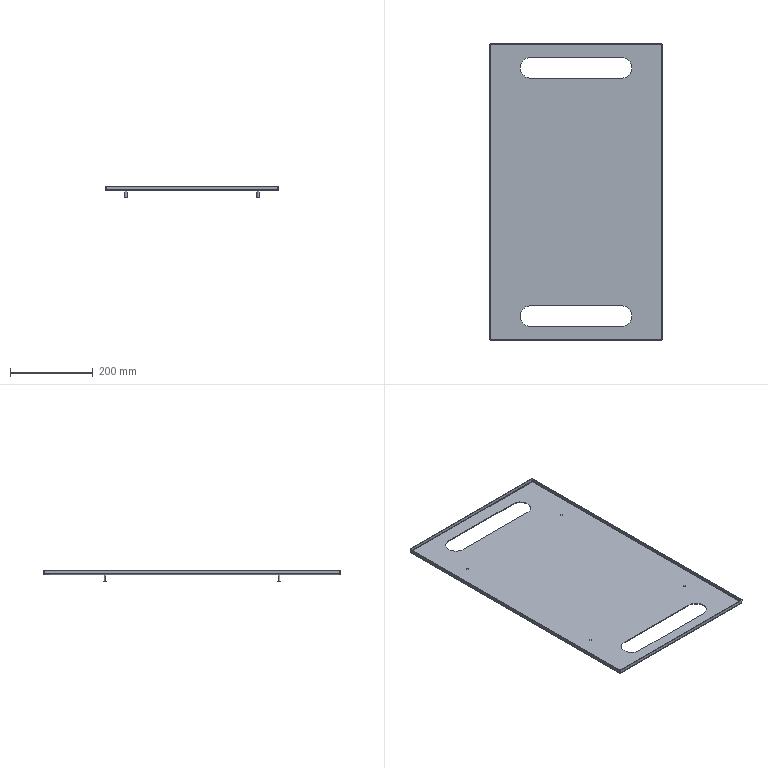Part | SolidWorks | features BaseBody 1 | 1 solid | 60 faces | box 420 x 720 x 25 mm | volume 587350 mm3 | plane 30 | cylinder 22 | spline 8 | commonest cylinder face diameters 6 x8 50 x6 1.473 x4 5.473 x4